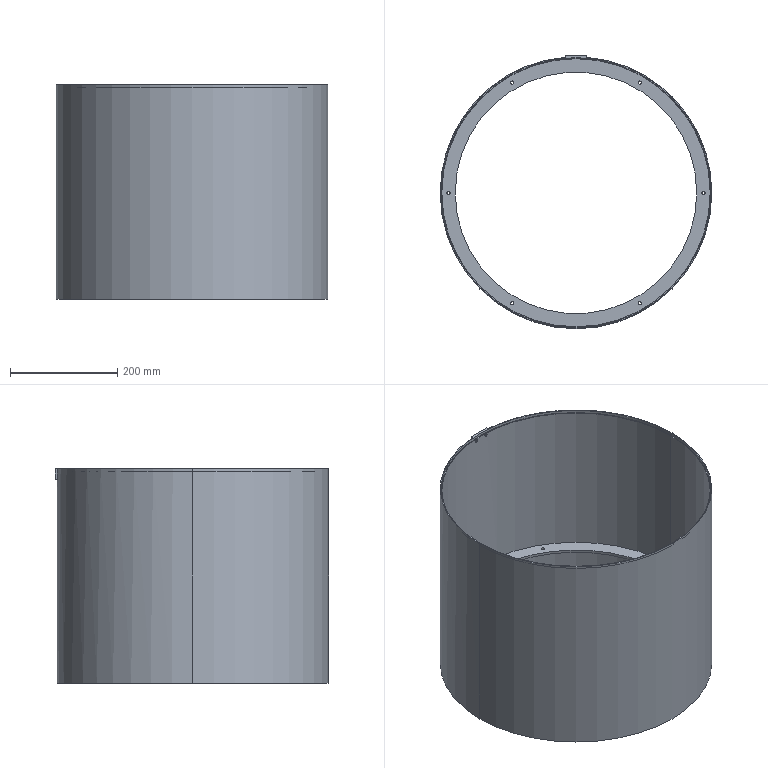Part | SolidWorks | features ICE 6, CirPattern 1, Extrusion 1 | 1 solid | 35 faces | box 506 x 509 x 400 mm | volume 2072487 mm3 | cylinder 26 | plane 9 | commonest cylinder face diameters 6 x12 5.21 x4 500 x4 450 x2 503 x2 506 x2
STEP:
#1=CARTESIAN_POINT('',(-251.5,0.,395.));
#2=VERTEX_POINT('',#1);
#3=CARTESIAN_POINT('',(251.5,0.,395.));
#4=VERTEX_POINT('',#3);
#5=CARTESIAN_POINT('',(0.,0.,395.));
#6=DIRECTION('',(0.,0.,1.));
#7=DIRECTION('',(1.,0.,0.));
#8=AXIS2_PLACEMENT_3D('',#5,#6,#7);
#9=CIRCLE('',#8,251.5);
#10=EDGE_CURVE('',#2,#4,#9,.T.);
#11=ORIENTED_EDGE('',*,*,#10,.F.);
#12=CARTESIAN_POINT('',(-251.5,0.,400.));
#13=VERTEX_POINT('',#12);
#14=CARTESIAN_POINT('',(-251.5,0.,395.));
#15=DIRECTION('',(0.,0.,1.));
#16=VECTOR('',#15,1000.);
#17=LINE('',#14,#16);
#18=EDGE_CURVE('',#2,#13,#17,.T.);
#19=ORIENTED_EDGE('',*,*,#18,.T.);
#20=CARTESIAN_POINT('',(251.5,0.,400.));
#21=VERTEX_POINT('',#20);
#22=CARTESIAN_POINT('',(0.,0.,400.));
#23=DIRECTION('',(0.,0.,1.));
#24=DIRECTION('',(1.,0.,0.));
#25=AXIS2_PLACEMENT_3D('',#22,#23,#24);
#26=CIRCLE('',#25,251.5);
#27=EDGE_CURVE('',#13,#21,#26,.T.);
#28=ORIENTED_EDGE('',*,*,#27,.T.);
#29=CARTESIAN_POINT('',(251.5,0.,395.));
#30=DIRECTION('',(0.,0.,1.));
#31=VECTOR('',#30,1000.);
#32=LINE('',#29,#31);
#33=EDGE_CURVE('',#4,#21,#32,.T.);
#34=ORIENTED_EDGE('',*,*,#33,.F.);
#35=EDGE_LOOP('',(#11,#19,#28,#34));
#36=FACE_OUTER_BOUND('',#35,.T.);
#37=CARTESIAN_POINT('',(0.,0.,395.));
#38=DIRECTION('',(0.,0.,1.));
#39=DIRECTION('',(1.,0.,0.));
#40=AXIS2_PLACEMENT_3D('',#37,#38,#39);
#41=CYLINDRICAL_SURFACE('',#40,251.5);
#42=ADVANCED_FACE('',(#36),#41,.F.);
#43=CARTESIAN_POINT('',(12.5,249.687,387.395));
#44=VERTEX_POINT('',#43);
#45=CARTESIAN_POINT('',(12.5,249.687,392.605));
#46=VERTEX_POINT('',#45);
#47=CARTESIAN_POINT('',(12.5,249.687,387.395));
#48=CARTESIAN_POINT('',(12.33,249.696,387.395));
#49=CARTESIAN_POINT('',(12.161,249.704,387.412));
#50=CARTESIAN_POINT('',(11.826,249.72,387.478));
#51=CARTESIAN_POINT('',(11.661,249.728,387.528));
#52=CARTESIAN_POINT('',(11.191,249.75,387.722));
#53=CARTESIAN_POINT('',(10.9,249.762,387.916));
#54=CARTESIAN_POINT('',(10.54,249.778,388.276));
#55=CARTESIAN_POINT('',(10.43,249.782,388.41));
#56=CARTESIAN_POINT('',(10.24,249.79,388.693));
#57=CARTESIAN_POINT('',(10.16,249.793,388.843));
#58=CARTESIAN_POINT('',(10.029,249.799,389.158));
#59=CARTESIAN_POINT('',(9.979,249.801,389.324));
#60=CARTESIAN_POINT('',(9.912,249.803,389.657));
#61=CARTESIAN_POINT('',(9.895,249.804,389.826));
#62=CARTESIAN_POINT('',(9.895,249.804,390.17));
#63=CARTESIAN_POINT('',(9.912,249.803,390.34));
#64=CARTESIAN_POINT('',(9.978,249.801,390.673));
#65=CARTESIAN_POINT('',(10.028,249.799,390.838));
#66=CARTESIAN_POINT('',(10.158,249.794,391.154));
#67=CARTESIAN_POINT('',(10.238,249.79,391.304));
#68=CARTESIAN_POINT('',(10.427,249.782,391.587));
#69=CARTESIAN_POINT('',(10.537,249.778,391.721));
#70=CARTESIAN_POINT('',(10.777,249.768,391.961));
#71=CARTESIAN_POINT('',(10.908,249.762,392.069));
#72=CARTESIAN_POINT('',(11.193,249.749,392.26));
#73=CARTESIAN_POINT('',(11.345,249.743,392.341));
#74=CARTESIAN_POINT('',(11.814,249.721,392.536));
#75=CARTESIAN_POINT('',(12.156,249.705,392.605));
#76=CARTESIAN_POINT('',(12.5,249.687,392.605));
#77=B_SPLINE_CURVE_WITH_KNOTS('',3,(#47,#48,#49,#50,#51,#52,#53,#54,#55,#56,#57,#58,#59,#60,#61,#62,#63,#64,#65,#66,#67,#68,#69,#70,#71,#72,#73,#74,#75,#76),.UNSPECIFIED.,.F.,.F.,(4,2,2,2,2,2,2,2,2,2,2,2,2,2,4),(0.00815,0.008659,0.009168,0.01019,0.0107,0.01121,0.01171,0.01222,0.01273,0.01324,0.01375,0.01426,0.01477,0.01528,0.0163),.UNSPECIFIED.);
#78=EDGE_CURVE('',#44,#46,#77,.T.);
#79=ORIENTED_EDGE('',*,*,#78,.F.);
#80=CARTESIAN_POINT('',(12.5,256.,387.395));
#81=VERTEX_POINT('',#80);
#82=CARTESIAN_POINT('',(12.5,-253.001,387.395));
#83=DIRECTION('',(0.,1.,0.));
#84=VECTOR('',#83,1000.);
#85=LINE('',#82,#84);
#86=EDGE_CURVE('',#44,#81,#85,.T.);
#87=ORIENTED_EDGE('',*,*,#86,.T.);
#88=CARTESIAN_POINT('',(12.5,256.,392.605));
#89=VERTEX_POINT('',#88);
#90=CARTESIAN_POINT('',(12.5,256.,390.));
#91=DIRECTION('',(0.,1.,0.));
#92=DIRECTION('',(0.,0.,-1.));
#93=AXIS2_PLACEMENT_3D('',#90,#91,#92);
#94=CIRCLE('',#93,2.605);
#95=EDGE_CURVE('',#81,#89,#94,.T.);
#96=ORIENTED_EDGE('',*,*,#95,.T.);
#97=CARTESIAN_POINT('',(12.5,-253.001,392.605));
#98=DIRECTION('',(0.,1.,0.));
#99=VECTOR('',#98,1000.);
#100=LINE('',#97,#99);
#101=EDGE_CURVE('',#46,#89,#100,.T.);
#102=ORIENTED_EDGE('',*,*,#101,.F.);
#103=EDGE_LOOP('',(#79,#87,#96,#102));
#104=FACE_OUTER_BOUND('',#103,.T.);
#105=CARTESIAN_POINT('',(12.5,-253.001,390.));
#106=DIRECTION('',(0.,1.,0.));
#107=DIRECTION('',(0.,0.,1.));
#108=AXIS2_PLACEMENT_3D('',#105,#106,#107);
#109=CYLINDRICAL_SURFACE('',#108,2.605);
#110=ADVANCED_FACE('',(#104),#109,.F.);
#111=CARTESIAN_POINT('',(-12.5,249.687,387.395));
#112=VERTEX_POINT('',#111);
#113=CARTESIAN_POINT('',(-12.5,249.687,392.605));
#114=VERTEX_POINT('',#113);
#115=CARTESIAN_POINT('',(-12.5,249.687,387.395));
#116=CARTESIAN_POINT('',(-12.67,249.679,387.395));
#117=CARTESIAN_POINT('',(-12.839,249.67,387.412));
#118=CARTESIAN_POINT('',(-13.174,249.653,387.478));
#119=CARTESIAN_POINT('',(-13.339,249.644,387.528));
#120=CARTESIAN_POINT('',(-13.809,249.619,387.722));
#121=CARTESIAN_POINT('',(-14.1,249.602,387.916));
#122=CARTESIAN_POINT('',(-14.46,249.581,388.276));
#123=CARTESIAN_POINT('',(-14.57,249.575,388.41));
#124=CARTESIAN_POINT('',(-14.76,249.564,388.693));
#125=CARTESIAN_POINT('',(-14.84,249.559,388.843));
#126=CARTESIAN_POINT('',(-14.971,249.551,389.158));
#127=CARTESIAN_POINT('',(-15.021,249.548,389.323));
#128=CARTESIAN_POINT('',(-15.088,249.544,389.657));
#129=CARTESIAN_POINT('',(-15.105,249.543,389.826));
#130=CARTESIAN_POINT('',(-15.105,249.543,390.17));
#131=CARTESIAN_POINT('',(-15.088,249.544,390.34));
#132=CARTESIAN_POINT('',(-15.022,249.548,390.673));
#133=CARTESIAN_POINT('',(-14.972,249.551,390.838));
#134=CARTESIAN_POINT('',(-14.842,249.559,391.154));
#135=CARTESIAN_POINT('',(-14.762,249.564,391.304));
#136=CARTESIAN_POINT('',(-14.573,249.575,391.587));
#137=CARTESIAN_POINT('',(-14.463,249.581,391.721));
#138=CARTESIAN_POINT('',(-14.222,249.595,391.962));
#139=CARTESIAN_POINT('',(-14.091,249.603,392.069));
#140=CARTESIAN_POINT('',(-13.807,249.618,392.26));
#141=CARTESIAN_POINT('',(-13.655,249.627,392.341));
#142=CARTESIAN_POINT('',(-13.186,249.652,392.536));
#143=CARTESIAN_POINT('',(-12.844,249.67,392.605));
#144=CARTESIAN_POINT('',(-12.5,249.687,392.605));
#145=B_SPLINE_CURVE_WITH_KNOTS('',3,(#115,#116,#117,#118,#119,#120,#121,#122,#123,#124,#125,#126,#127,#128,#129,#130,#131,#132,#133,#134,#135,#136,#137,#138,#139,#140,#141,#142,#143,#144),.UNSPECIFIED.,.F.,.F.,(4,2,2,2,2,2,2,2,2,2,2,2,2,2,4),(0.008148,0.008658,0.009167,0.01019,0.01069,0.0112,0.01171,0.01222,0.01273,0.01324,0.01375,0.01426,0.01477,0.01528,0.0163),.UNSPECIFIED.);
#146=EDGE_CURVE('',#112,#114,#145,.T.);
#147=ORIENTED_EDGE('',*,*,#146,.F.);
#148=CARTESIAN_POINT('',(-12.5,256.,387.395));
#149=VERTEX_POINT('',#148);
#150=CARTESIAN_POINT('',(-12.5,-253.001,387.395));
#151=DIRECTION('',(0.,1.,0.));
#152=VECTOR('',#151,1000.);
#153=LINE('',#150,#152);
#154=EDGE_CURVE('',#112,#149,#153,.T.);
#155=ORIENTED_EDGE('',*,*,#154,.T.);
#156=CARTESIAN_POINT('',(-12.5,256.,392.605));
#157=VERTEX_POINT('',#156);
#158=CARTESIAN_POINT('',(-12.5,256.,390.));
#159=DIRECTION('',(0.,1.,0.));
#160=DIRECTION('',(0.,0.,1.));
#161=AXIS2_PLACEMENT_3D('',#158,#159,#160);
#162=CIRCLE('',#161,2.605);
#163=EDGE_CURVE('',#149,#157,#162,.T.);
#164=ORIENTED_EDGE('',*,*,#163,.T.);
#165=CARTESIAN_POINT('',(-12.5,-253.001,392.605));
#166=DIRECTION('',(0.,1.,0.));
#167=VECTOR('',#166,1000.);
#168=LINE('',#165,#167);
#169=EDGE_CURVE('',#114,#157,#168,.T.);
#170=ORIENTED_EDGE('',*,*,#169,.F.);
#171=EDGE_LOOP('',(#147,#155,#164,#170));
#172=FACE_OUTER_BOUND('',#171,.T.);
#173=CARTESIAN_POINT('',(-12.5,-253.001,390.));
#174=DIRECTION('',(0.,1.,0.));
#175=DIRECTION('',(0.,0.,1.));
#176=AXIS2_PLACEMENT_3D('',#173,#174,#175);
#177=CYLINDRICAL_SURFACE('',#176,2.605);
#178=ADVANCED_FACE('',(#172),#177,.F.);
#179=CARTESIAN_POINT('',(121.75,205.681,100.));
#180=VERTEX_POINT('',#179);
#181=CARTESIAN_POINT('',(115.75,205.681,100.));
#182=VERTEX_POINT('',#181);
#183=CARTESIAN_POINT('',(118.75,205.681,100.));
#184=DIRECTION('',(0.,0.,-1.));
#185=DIRECTION('',(-1.,0.,0.));
#186=AXIS2_PLACEMENT_3D('',#183,#184,#185);
#187=CIRCLE('',#186,3.);
#188=EDGE_CURVE('',#180,#182,#187,.T.);
#189=ORIENTED_EDGE('',*,*,#188,.F.);
#190=CARTESIAN_POINT('',(121.75,205.681,95.));
#191=VERTEX_POINT('',#190);
#192=CARTESIAN_POINT('',(121.75,205.681,115.));
#193=DIRECTION('',(0.,0.,-1.));
#194=VECTOR('',#193,1000.);
#195=LINE('',#192,#194);
#196=EDGE_CURVE('',#180,#191,#195,.T.);
#197=ORIENTED_EDGE('',*,*,#196,.T.);
#198=CARTESIAN_POINT('',(115.75,205.681,95.));
#199=VERTEX_POINT('',#198);
#200=CARTESIAN_POINT('',(118.75,205.681,95.));
#201=DIRECTION('',(0.,0.,-1.));
#202=DIRECTION('',(0.5,0.866,0.));
#203=AXIS2_PLACEMENT_3D('',#200,#201,#202);
#204=CIRCLE('',#203,3.);
#205=EDGE_CURVE('',#191,#199,#204,.T.);
#206=ORIENTED_EDGE('',*,*,#205,.T.);
#207=CARTESIAN_POINT('',(115.75,205.681,115.));
#208=DIRECTION('',(0.,0.,-1.));
#209=VECTOR('',#208,1000.);
#210=LINE('',#207,#209);
#211=EDGE_CURVE('',#182,#199,#210,.T.);
#212=ORIENTED_EDGE('',*,*,#211,.F.);
#213=EDGE_LOOP('',(#189,#197,#206,#212));
#214=FACE_OUTER_BOUND('',#213,.T.);
#215=CARTESIAN_POINT('',(118.75,205.681,115.));
#216=DIRECTION('',(0.,0.,-1.));
#217=DIRECTION('',(-1.,0.,0.));
#218=AXIS2_PLACEMENT_3D('',#215,#216,#217);
#219=CYLINDRICAL_SURFACE('',#218,3.);
#220=ADVANCED_FACE('',(#214),#219,.F.);
#221=CARTESIAN_POINT('',(240.5,0.,100.));
#222=VERTEX_POINT('',#221);
#223=CARTESIAN_POINT('',(234.5,0.,100.));
#224=VERTEX_POINT('',#223);
#225=CARTESIAN_POINT('',(237.5,0.,100.));
#226=DIRECTION('',(0.,0.,-1.));
#227=DIRECTION('',(-1.,0.,0.));
#228=AXIS2_PLACEMENT_3D('',#225,#226,#227);
#229=CIRCLE('',#228,3.);
#230=EDGE_CURVE('',#222,#224,#229,.T.);
#231=ORIENTED_EDGE('',*,*,#230,.F.);
#232=CARTESIAN_POINT('',(240.5,0.,95.));
#233=VERTEX_POINT('',#232);
#234=CARTESIAN_POINT('',(240.5,0.,115.));
#235=DIRECTION('',(0.,0.,-1.));
#236=VECTOR('',#235,1000.);
#237=LINE('',#234,#236);
#238=EDGE_CURVE('',#222,#233,#237,.T.);
#239=ORIENTED_EDGE('',*,*,#238,.T.);
#240=CARTESIAN_POINT('',(234.5,0.,95.));
#241=VERTEX_POINT('',#240);
#242=CARTESIAN_POINT('',(237.5,0.,95.));
#243=DIRECTION('',(0.,0.,-1.));
#244=DIRECTION('',(1.,0.,0.));
#245=AXIS2_PLACEMENT_3D('',#242,#243,#244);
#246=CIRCLE('',#245,3.);
#247=EDGE_CURVE('',#233,#241,#246,.T.);
#248=ORIENTED_EDGE('',*,*,#247,.T.);
#249=CARTESIAN_POINT('',(234.5,0.,115.));
#250=DIRECTION('',(0.,0.,-1.));
#251=VECTOR('',#250,1000.);
#252=LINE('',#249,#251);
#253=EDGE_CURVE('',#224,#241,#252,.T.);
#254=ORIENTED_EDGE('',*,*,#253,.F.);
#255=EDGE_LOOP('',(#231,#239,#248,#254));
#256=FACE_OUTER_BOUND('',#255,.T.);
#257=CARTESIAN_POINT('',(237.5,0.,115.));
#258=DIRECTION('',(0.,0.,-1.));
#259=DIRECTION('',(-1.,0.,0.));
#260=AXIS2_PLACEMENT_3D('',#257,#258,#259);
#261=CYLINDRICAL_SURFACE('',#260,3.);
#262=ADVANCED_FACE('',(#256),#261,.F.);
#263=CARTESIAN_POINT('',(121.75,-205.681,100.));
#264=VERTEX_POINT('',#263);
#265=CARTESIAN_POINT('',(115.75,-205.681,100.));
#266=VERTEX_POINT('',#265);
#267=CARTESIAN_POINT('',(118.75,-205.681,100.));
#268=DIRECTION('',(0.,0.,-1.));
#269=DIRECTION('',(-1.,0.,0.));
#270=AXIS2_PLACEMENT_3D('',#267,#268,#269);
#271=CIRCLE('',#270,3.);
#272=EDGE_CURVE('',#264,#266,#271,.T.);
#273=ORIENTED_EDGE('',*,*,#272,.F.);
#274=CARTESIAN_POINT('',(121.75,-205.681,95.));
#275=VERTEX_POINT('',#274);
#276=CARTESIAN_POINT('',(121.75,-205.681,115.));
#277=DIRECTION('',(0.,0.,-1.));
#278=VECTOR('',#277,1000.);
#279=LINE('',#276,#278);
#280=EDGE_CURVE('',#264,#275,#279,.T.);
#281=ORIENTED_EDGE('',*,*,#280,.T.);
#282=CARTESIAN_POINT('',(115.75,-205.681,95.));
#283=VERTEX_POINT('',#282);
#284=CARTESIAN_POINT('',(118.75,-205.681,95.));
#285=DIRECTION('',(0.,0.,-1.));
#286=DIRECTION('',(0.5,-0.866,0.));
#287=AXIS2_PLACEMENT_3D('',#284,#285,#286);
#288=CIRCLE('',#287,3.);
#289=EDGE_CURVE('',#275,#283,#288,.T.);
#290=ORIENTED_EDGE('',*,*,#289,.T.);
#291=CARTESIAN_POINT('',(115.75,-205.681,115.));
#292=DIRECTION('',(0.,0.,-1.));
#293=VECTOR('',#292,1000.);
#294=LINE('',#291,#293);
#295=EDGE_CURVE('',#266,#283,#294,.T.);
#296=ORIENTED_EDGE('',*,*,#295,.F.);
#297=EDGE_LOOP('',(#273,#281,#290,#296));
#298=FACE_OUTER_BOUND('',#297,.T.);
#299=CARTESIAN_POINT('',(118.75,-205.681,115.));
#300=DIRECTION('',(0.,0.,-1.));
#301=DIRECTION('',(-1.,0.,0.));
#302=AXIS2_PLACEMENT_3D('',#299,#300,#301);
#303=CYLINDRICAL_SURFACE('',#302,3.);
#304=ADVANCED_FACE('',(#298),#303,.F.);
#305=CARTESIAN_POINT('',(-115.75,-205.681,100.));
#306=VERTEX_POINT('',#305);
#307=CARTESIAN_POINT('',(-121.75,-205.681,100.));
#308=VERTEX_POINT('',#307);
#309=CARTESIAN_POINT('',(-118.75,-205.681,100.));
#310=DIRECTION('',(0.,0.,-1.));
#311=DIRECTION('',(-1.,0.,0.));
#312=AXIS2_PLACEMENT_3D('',#309,#310,#311);
#313=CIRCLE('',#312,3.);
#314=EDGE_CURVE('',#306,#308,#313,.T.);
#315=ORIENTED_EDGE('',*,*,#314,.F.);
#316=CARTESIAN_POINT('',(-115.75,-205.681,95.));
#317=VERTEX_POINT('',#316);
#318=CARTESIAN_POINT('',(-115.75,-205.681,115.));
#319=DIRECTION('',(0.,0.,-1.));
#320=VECTOR('',#319,1000.);
#321=LINE('',#318,#320);
#322=EDGE_CURVE('',#306,#317,#321,.T.);
#323=ORIENTED_EDGE('',*,*,#322,.T.);
#324=CARTESIAN_POINT('',(-121.75,-205.681,95.));
#325=VERTEX_POINT('',#324);
#326=CARTESIAN_POINT('',(-118.75,-205.681,95.));
#327=DIRECTION('',(0.,0.,-1.));
#328=DIRECTION('',(-0.5,-0.866,0.));
#329=AXIS2_PLACEMENT_3D('',#326,#327,#328);
#330=CIRCLE('',#329,3.);
#331=EDGE_CURVE('',#317,#325,#330,.T.);
#332=ORIENTED_EDGE('',*,*,#331,.T.);
#333=CARTESIAN_POINT('',(-121.75,-205.681,115.));
#334=DIRECTION('',(0.,0.,-1.));
#335=VECTOR('',#334,1000.);
#336=LINE('',#333,#335);
#337=EDGE_CURVE('',#308,#325,#336,.T.);
#338=ORIENTED_EDGE('',*,*,#337,.F.);
#339=EDGE_LOOP('',(#315,#323,#332,#338));
#340=FACE_OUTER_BOUND('',#339,.T.);
#341=CARTESIAN_POINT('',(-118.75,-205.681,115.));
#342=DIRECTION('',(0.,0.,-1.));
#343=DIRECTION('',(-1.,0.,0.));
#344=AXIS2_PLACEMENT_3D('',#341,#342,#343);
#345=CYLINDRICAL_SURFACE('',#344,3.);
#346=ADVANCED_FACE('',(#340),#345,.F.);
#347=CARTESIAN_POINT('',(-115.75,205.681,100.));
#348=VERTEX_POINT('',#347);
#349=CARTESIAN_POINT('',(-121.75,205.681,100.));
#350=VERTEX_POINT('',#349);
#351=CARTESIAN_POINT('',(-118.75,205.681,100.));
#352=DIRECTION('',(0.,0.,-1.));
#353=DIRECTION('',(-1.,0.,0.));
#354=AXIS2_PLACEMENT_3D('',#351,#352,#353);
#355=CIRCLE('',#354,3.);
#356=EDGE_CURVE('',#348,#350,#355,.T.);
#357=ORIENTED_EDGE('',*,*,#356,.F.);
#358=CARTESIAN_POINT('',(-115.75,205.681,95.));
#359=VERTEX_POINT('',#358);
#360=CARTESIAN_POINT('',(-115.75,205.681,115.));
#361=DIRECTION('',(0.,0.,-1.));
#362=VECTOR('',#361,1000.);
#363=LINE('',#360,#362);
#364=EDGE_CURVE('',#348,#359,#363,.T.);
#365=ORIENTED_EDGE('',*,*,#364,.T.);
#366=CARTESIAN_POINT('',(-121.75,205.681,95.));
#367=VERTEX_POINT('',#366);
#368=CARTESIAN_POINT('',(-118.75,205.681,95.));
#369=DIRECTION('',(0.,0.,-1.));
#370=DIRECTION('',(-0.5,0.866,0.));
#371=AXIS2_PLACEMENT_3D('',#368,#369,#370);
#372=CIRCLE('',#371,3.);
#373=EDGE_CURVE('',#359,#367,#372,.T.);
#374=ORIENTED_EDGE('',*,*,#373,.T.);
#375=CARTESIAN_POINT('',(-121.75,205.681,115.));
#376=DIRECTION('',(0.,0.,-1.));
#377=VECTOR('',#376,1000.);
#378=LINE('',#375,#377);
#379=EDGE_CURVE('',#350,#367,#378,.T.);
#380=ORIENTED_EDGE('',*,*,#379,.F.);
#381=EDGE_LOOP('',(#357,#365,#374,#380));
#382=FACE_OUTER_BOUND('',#381,.T.);
#383=CARTESIAN_POINT('',(-118.75,205.681,115.));
#384=DIRECTION('',(0.,0.,-1.));
#385=DIRECTION('',(-1.,0.,0.));
#386=AXIS2_PLACEMENT_3D('',#383,#384,#385);
#387=CYLINDRICAL_SURFACE('',#386,3.);
#388=ADVANCED_FACE('',(#382),#387,.F.);
#389=CARTESIAN_POINT('',(-234.5,0.,100.));
#390=VERTEX_POINT('',#389);
#391=CARTESIAN_POINT('',(-240.5,0.,100.));
#392=VERTEX_POINT('',#391);
#393=CARTESIAN_POINT('',(-237.5,0.,100.));
#394=DIRECTION('',(0.,0.,-1.));
#395=DIRECTION('',(-1.,0.,0.));
#396=AXIS2_PLACEMENT_3D('',#393,#394,#395);
#397=CIRCLE('',#396,3.);
#398=EDGE_CURVE('',#390,#392,#397,.T.);
#399=ORIENTED_EDGE('',*,*,#398,.F.);
#400=CARTESIAN_POINT('',(-234.5,0.,95.));
#401=VERTEX_POINT('',#400);
#402=CARTESIAN_POINT('',(-234.5,0.,115.));
#403=DIRECTION('',(0.,0.,-1.));
#404=VECTOR('',#403,1000.);
#405=LINE('',#402,#404);
#406=EDGE_CURVE('',#390,#401,#405,.T.);
#407=ORIENTED_EDGE('',*,*,#406,.T.);
#408=CARTESIAN_POINT('',(-240.5,0.,95.));
#409=VERTEX_POINT('',#408);
#410=CARTESIAN_POINT('',(-237.5,0.,95.));
#411=DIRECTION('',(0.,0.,-1.));
#412=DIRECTION('',(-1.,0.,0.));
#413=AXIS2_PLACEMENT_3D('',#410,#411,#412);
#414=CIRCLE('',#413,3.);
#415=EDGE_CURVE('',#401,#409,#414,.T.);
#416=ORIENTED_EDGE('',*,*,#415,.T.);
#417=CARTESIAN_POINT('',(-240.5,0.,115.));
#418=DIRECTION('',(0.,0.,-1.));
#419=VECTOR('',#418,1000.);
#420=LINE('',#417,#419);
#421=EDGE_CURVE('',#392,#409,#420,.T.);
#422=ORIENTED_EDGE('',*,*,#421,.F.);
#423=EDGE_LOOP('',(#399,#407,#416,#422));
#424=FACE_OUTER_BOUND('',#423,.T.);
#425=CARTESIAN_POINT('',(-237.5,0.,115.));
#426=DIRECTION('',(0.,0.,-1.));
#427=DIRECTION('',(-1.,0.,0.));
#428=AXIS2_PLACEMENT_3D('',#425,#426,#427);
#429=CYLINDRICAL_SURFACE('',#428,3.);
#430=ADVANCED_FACE('',(#424),#429,.F.);
#431=CARTESIAN_POINT('',(225.,0.,95.));
#432=VERTEX_POINT('',#431);
#433=CARTESIAN_POINT('',(-225.,0.,95.));
#434=VERTEX_POINT('',#433);
#435=CARTESIAN_POINT('',(0.,0.,95.));
#436=DIRECTION('',(0.,0.,-1.));
#437=DIRECTION('',(-1.,0.,0.));
#438=AXIS2_PLACEMENT_3D('',#435,#436,#437);
#439=CIRCLE('',#438,225.);
#440=EDGE_CURVE('',#432,#434,#439,.T.);
#441=ORIENTED_EDGE('',*,*,#440,.T.);
#442=CARTESIAN_POINT('',(-225.,0.,100.));
#443=VERTEX_POINT('',#442);
#444=CARTESIAN_POINT('',(-225.,0.,95.));
#445=DIRECTION('',(0.,0.,1.));
#446=VECTOR('',#445,1000.);
#447=LINE('',#444,#446);
#448=EDGE_CURVE('',#434,#443,#447,.T.);
#449=ORIENTED_EDGE('',*,*,#448,.T.);
#450=CARTESIAN_POINT('',(225.,0.,100.));
#451=VERTEX_POINT('',#450);
#452=CARTESIAN_POINT('',(0.,0.,100.));
#453=DIRECTION('',(0.,0.,-1.));
#454=DIRECTION('',(-1.,0.,0.));
#455=AXIS2_PLACEMENT_3D('',#452,#453,#454);
#456=CIRCLE('',#455,225.);
#457=EDGE_CURVE('',#451,#443,#456,.T.);
#458=ORIENTED_EDGE('',*,*,#457,.F.);
#459=CARTESIAN_POINT('',(225.,0.,95.));
#460=DIRECTION('',(0.,0.,1.));
#461=VECTOR('',#460,1000.);
#462=LINE('',#459,#461);
#463=EDGE_CURVE('',#432,#451,#462,.T.);
#464=ORIENTED_EDGE('',*,*,#463,.F.);
#465=EDGE_LOOP('',(#441,#449,#458,#464));
#466=FACE_OUTER_BOUND('',#465,.T.);
#467=CARTESIAN_POINT('',(0.,0.,95.));
#468=DIRECTION('',(0.,0.,1.));
#469=DIRECTION('',(1.,0.,0.));
#470=AXIS2_PLACEMENT_3D('',#467,#468,#469);
#471=CYLINDRICAL_SURFACE('',#470,225.);
#472=ADVANCED_FACE('',(#466),#471,.F.);
#473=CARTESIAN_POINT('',(250.,0.,95.));
#474=VERTEX_POINT('',#473);
#475=CARTESIAN_POINT('',(-250.,0.,95.));
#476=VERTEX_POINT('',#475);
#477=CARTESIAN_POINT('',(0.,0.,95.));
#478=DIRECTION('',(0.,0.,-1.));
#479=DIRECTION('',(-1.,0.,0.));
#480=AXIS2_PLACEMENT_3D('',#477,#478,#479);
#481=CIRCLE('',#480,250.);
#482=EDGE_CURVE('',#474,#476,#481,.T.);
#483=ORIENTED_EDGE('',*,*,#482,.F.);
#484=CARTESIAN_POINT('',(250.,0.,0.));
#485=VERTEX_POINT('',#484);
#486=CARTESIAN_POINT('',(250.,0.,400.));
#487=DIRECTION('',(0.,0.,-1.));
#488=VECTOR('',#487,1000.);
#489=LINE('',#486,#488);
#490=EDGE_CURVE('',#474,#485,#489,.T.);
#491=ORIENTED_EDGE('',*,*,#490,.T.);
#492=CARTESIAN_POINT('',(-250.,0.,0.));
#493=VERTEX_POINT('',#492);
#494=CARTESIAN_POINT('',(0.,0.,0.));
#495=DIRECTION('',(0.,0.,1.));
#496=DIRECTION('',(1.,0.,0.));
#497=AXIS2_PLACEMENT_3D('',#494,#495,#496);
#498=CIRCLE('',#497,250.);
#499=EDGE_CURVE('',#493,#485,#498,.T.);
#500=ORIENTED_EDGE('',*,*,#499,.F.);
#501=CARTESIAN_POINT('',(-250.,0.,400.));
#502=DIRECTION('',(0.,0.,-1.));
#503=VECTOR('',#502,1000.);
#504=LINE('',#501,#503);
#505=EDGE_CURVE('',#476,#493,#504,.T.);
#506=ORIENTED_EDGE('',*,*,#505,.F.);
#507=EDGE_LOOP('',(#483,#491,#500,#506));
#508=FACE_OUTER_BOUND('',#507,.T.);
#509=CARTESIAN_POINT('',(0.,0.,400.));
#510=DIRECTION('',(0.,0.,-1.));
#511=DIRECTION('',(-1.,0.,0.));
#512=AXIS2_PLACEMENT_3D('',#509,#510,#511);
#513=CYLINDRICAL_SURFACE('',#512,250.);
#514=ADVANCED_FACE('',(#508),#513,.F.);
#515=CARTESIAN_POINT('',(253.,0.,400.));
#516=VERTEX_POINT('',#515);
#517=CARTESIAN_POINT('',(20.,252.208,400.));
#518=VERTEX_POINT('',#517);
#519=CARTESIAN_POINT('',(0.,0.,400.));
#520=DIRECTION('',(0.,0.,1.));
#521=DIRECTION('',(1.,0.,0.));
#522=AXIS2_PLACEMENT_3D('',#519,#520,#521);
#523=CIRCLE('',#522,253.);
#524=EDGE_CURVE('',#516,#518,#523,.T.);
#525=ORIENTED_EDGE('',*,*,#524,.F.);
#526=CARTESIAN_POINT('',(253.,0.,0.));
#527=VERTEX_POINT('',#526);
#528=CARTESIAN_POINT('',(253.,0.,400.));
#529=DIRECTION('',(0.,0.,-1.));
#530=VECTOR('',#529,1000.);
#531=LINE('',#528,#530);
#532=EDGE_CURVE('',#516,#527,#531,.T.);
#533=ORIENTED_EDGE('',*,*,#532,.T.);
#534=CARTESIAN_POINT('',(-253.,0.,0.));
#535=VERTEX_POINT('',#534);
#536=CARTESIAN_POINT('',(0.,0.,0.));
#537=DIRECTION('',(0.,0.,1.));
#538=DIRECTION('',(1.,0.,0.));
#539=AXIS2_PLACEMENT_3D('',#536,#537,#538);
#540=CIRCLE('',#539,253.);
#541=EDGE_CURVE('',#527,#535,#540,.T.);
#542=ORIENTED_EDGE('',*,*,#541,.T.);
#543=CARTESIAN_POINT('',(-253.,0.,400.));
#544=VERTEX_POINT('',#543);
#545=CARTESIAN_POINT('',(-253.,0.,400.));
#546=DIRECTION('',(0.,0.,-1.));
#547=VECTOR('',#546,1000.);
#548=LINE('',#545,#547);
#549=EDGE_CURVE('',#544,#535,#548,.T.);
#550=ORIENTED_EDGE('',*,*,#549,.F.);
#551=CARTESIAN_POINT('',(-20.,252.208,400.));
#552=VERTEX_POINT('',#551);
#553=CARTESIAN_POINT('',(0.,0.,400.));
#554=DIRECTION('',(0.,0.,1.));
#555=DIRECTION('',(1.,0.,0.));
#556=AXIS2_PLACEMENT_3D('',#553,#554,#555);
#557=CIRCLE('',#556,253.);
#558=EDGE_CURVE('',#552,#544,#557,.T.);
#559=ORIENTED_EDGE('',*,*,#558,.F.);
#560=CARTESIAN_POINT('',(-20.,252.208,380.));
#561=VERTEX_POINT('',#560);
#562=CARTESIAN_POINT('',(-20.,252.208,400.));
#563=DIRECTION('',(0.,0.,1.));
#564=VECTOR('',#563,1000.);
#565=LINE('',#562,#564);
#566=EDGE_CURVE('',#561,#552,#565,.T.);
#567=ORIENTED_EDGE('',*,*,#566,.F.);
#568=CARTESIAN_POINT('',(20.,252.208,380.));
#569=VERTEX_POINT('',#568);
#570=CARTESIAN_POINT('',(0.,0.,380.));
#571=DIRECTION('',(0.,0.,1.));
#572=DIRECTION('',(-1.,0.,0.));
#573=AXIS2_PLACEMENT_3D('',#570,#571,#572);
#574=CIRCLE('',#573,253.);
#575=EDGE_CURVE('',#569,#561,#574,.T.);
#576=ORIENTED_EDGE('',*,*,#575,.F.);
#577=CARTESIAN_POINT('',(20.,252.208,400.));
#578=DIRECTION('',(0.,0.,-1.));
#579=VECTOR('',#578,1000.);
#580=LINE('',#577,#579);
#581=EDGE_CURVE('',#518,#569,#580,.T.);
#582=ORIENTED_EDGE('',*,*,#581,.F.);
#583=EDGE_LOOP('',(#525,#533,#542,#550,#559,#567,#576,#582));
#584=FACE_OUTER_BOUND('',#583,.T.);
#585=CARTESIAN_POINT('',(0.,0.,400.));
#586=DIRECTION('',(0.,0.,-1.));
#587=DIRECTION('',(-1.,0.,0.));
#588=AXIS2_PLACEMENT_3D('',#585,#586,#587);
#589=CYLINDRICAL_SURFACE('',#588,253.);
#590=ADVANCED_FACE('',(#584),#589,.T.);
#591=CARTESIAN_POINT('',(-250.,0.,395.));
#592=VERTEX_POINT('',#591);
#593=CARTESIAN_POINT('',(250.,0.,395.));
#594=VERTEX_POINT('',#593);
#595=CARTESIAN_POINT('',(0.,0.,395.));
#596=DIRECTION('',(0.,0.,1.));
#597=DIRECTION('',(1.,0.,0.));
#598=AXIS2_PLACEMENT_3D('',#595,#596,#597);
#599=CIRCLE('',#598,250.);
#600=EDGE_CURVE('',#592,#594,#599,.T.);
#601=ORIENTED_EDGE('',*,*,#600,.T.);
#602=CARTESIAN_POINT('',(250.,0.,100.));
#603=VERTEX_POINT('',#602);
#604=CARTESIAN_POINT('',(250.,0.,400.));
#605=DIRECTION('',(0.,0.,-1.));
#606=VECTOR('',#605,1000.);
#607=LINE('',#604,#606);
#608=EDGE_CURVE('',#594,#603,#607,.T.);
#609=ORIENTED_EDGE('',*,*,#608,.T.);
#610=CARTESIAN_POINT('',(-250.,0.,100.));
#611=VERTEX_POINT('',#610);
#612=CARTESIAN_POINT('',(0.,0.,100.));
#613=DIRECTION('',(0.,0.,-1.));
#614=DIRECTION('',(-1.,0.,0.));
#615=AXIS2_PLACEMENT_3D('',#612,#613,#614);
#616=CIRCLE('',#615,250.);
#617=EDGE_CURVE('',#603,#611,#616,.T.);
#618=ORIENTED_EDGE('',*,*,#617,.T.);
#619=CARTESIAN_POINT('',(-250.,0.,400.));
#620=DIRECTION('',(0.,0.,-1.));
#621=VECTOR('',#620,1000.);
#622=LINE('',#619,#621);
#623=EDGE_CURVE('',#592,#611,#622,.T.);
#624=ORIENTED_EDGE('',*,*,#623,.F.);
#625=EDGE_LOOP('',(#601,#609,#618,#624));
#626=FACE_OUTER_BOUND('',#625,.T.);
#627=CARTESIAN_POINT('',(0.,0.,400.));
#628=DIRECTION('',(0.,0.,-1.));
#629=DIRECTION('',(-1.,0.,0.));
#630=AXIS2_PLACEMENT_3D('',#627,#628,#629);
#631=CYLINDRICAL_SURFACE('',#630,250.);
#632=ADVANCED_FACE('',(#626),#631,.F.);
#633=ORIENTED_EDGE('',*,*,#608,.F.);
#634=CARTESIAN_POINT('',(0.,0.,395.));
#635=DIRECTION('',(0.,0.,1.));
#636=DIRECTION('',(1.,0.,0.));
#637=AXIS2_PLACEMENT_3D('',#634,#635,#636);
#638=CIRCLE('',#637,250.);
#639=EDGE_CURVE('',#594,#592,#638,.T.);
#640=ORIENTED_EDGE('',*,*,#639,.T.);
#641=ORIENTED_EDGE('',*,*,#623,.T.);
#642=CARTESIAN_POINT('',(0.,0.,100.));
#643=DIRECTION('',(0.,0.,-1.));
#644=DIRECTION('',(-1.,0.,0.));
#645=AXIS2_PLACEMENT_3D('',#642,#643,#644);
#646=CIRCLE('',#645,250.);
#647=EDGE_CURVE('',#611,#603,#646,.T.);
#648=ORIENTED_EDGE('',*,*,#647,.T.);
#649=EDGE_LOOP('',(#633,#640,#641,#648));
#650=FACE_OUTER_BOUND('',#649,.T.);
#651=CARTESIAN_POINT('',(-12.5,249.687,392.605));
#652=CARTESIAN_POINT('',(-12.328,249.696,392.605));
#653=CARTESIAN_POINT('',(-12.159,249.704,392.588));
#654=CARTESIAN_POINT('',(-11.826,249.72,392.522));
#655=CARTESIAN_POINT('',(-11.661,249.728,392.472));
#656=CARTESIAN_POINT('',(-11.345,249.742,392.341));
#657=CARTESIAN_POINT('',(-11.196,249.749,392.261));
#658=CARTESIAN_POINT('',(-10.913,249.762,392.072));
#659=CARTESIAN_POINT('',(-10.778,249.768,391.962));
#660=CARTESIAN_POINT('',(-10.538,249.778,391.722));
#661=CARTESIAN_POINT('',(-10.43,249.782,391.591));
#662=CARTESIAN_POINT('',(-10.24,249.79,391.306));
#663=CARTESIAN_POINT('',(-10.159,249.794,391.154));
#664=CARTESIAN_POINT('',(-10.029,249.799,390.841));
#665=CARTESIAN_POINT('',(-9.979,249.801,390.677));
#666=CARTESIAN_POINT('',(-9.912,249.803,390.34));
#667=CARTESIAN_POINT('',(-9.895,249.804,390.171));
#668=CARTESIAN_POINT('',(-9.895,249.804,389.831));
#669=CARTESIAN_POINT('',(-9.912,249.803,389.658));
#670=CARTESIAN_POINT('',(-9.979,249.801,389.324));
#671=CARTESIAN_POINT('',(-10.028,249.799,389.162));
#672=CARTESIAN_POINT('',(-10.158,249.794,388.846));
#673=CARTESIAN_POINT('',(-10.24,249.79,388.693));
#674=CARTESIAN_POINT('',(-10.429,249.782,388.411));
#675=CARTESIAN_POINT('',(-10.537,249.778,388.28));
#676=CARTESIAN_POINT('',(-10.78,249.768,388.036));
#677=CARTESIAN_POINT('',(-10.912,249.762,387.928));
#678=CARTESIAN_POINT('',(-11.194,249.749,387.74));
#679=CARTESIAN_POINT('',(-11.346,249.742,387.658));
#680=CARTESIAN_POINT('',(-11.662,249.728,387.528));
#681=CARTESIAN_POINT('',(-11.824,249.72,387.479));
#682=CARTESIAN_POINT('',(-12.158,249.704,387.412));
#683=CARTESIAN_POINT('',(-12.33,249.696,387.395));
#684=CARTESIAN_POINT('',(-12.5,249.687,387.395));
#685=B_SPLINE_CURVE_WITH_KNOTS('',3,(#651,#652,#653,#654,#655,#656,#657,#658,#659,#660,#661,#662,#663,#664,#665,#666,#667,#668,#669,#670,#671,#672,#673,#674,#675,#676,#677,#678,#679,#680,#681,#682,#683,#684),.UNSPECIFIED.,.F.,.F.,(4,2,2,2,2,2,2,2,2,2,2,2,2,2,2,2,4),(0.,0.0005093,0.001019,0.001528,0.002037,0.002546,0.003056,0.003565,0.004074,0.004583,0.005093,0.005602,0.006111,0.006621,0.00713,0.007639,0.008148),.UNSPECIFIED.);
#686=EDGE_CURVE('',#114,#112,#685,.T.);
#687=ORIENTED_EDGE('',*,*,#686,.T.);
#688=ORIENTED_EDGE('',*,*,#146,.T.);
#689=EDGE_LOOP('',(#687,#688));
#690=FACE_BOUND('',#689,.T.);
#691=CARTESIAN_POINT('',(12.5,249.687,392.605));
#692=CARTESIAN_POINT('',(12.672,249.679,392.605));
#693=CARTESIAN_POINT('',(12.841,249.67,392.588));
#694=CARTESIAN_POINT('',(13.174,249.653,392.522));
#695=CARTESIAN_POINT('',(13.339,249.644,392.472));
#696=CARTESIAN_POINT('',(13.655,249.627,392.341));
#697=CARTESIAN_POINT('',(13.804,249.619,392.261));
#698=CARTESIAN_POINT('',(14.087,249.603,392.072));
#699=CARTESIAN_POINT('',(14.221,249.595,391.962));
#700=CARTESIAN_POINT('',(14.462,249.581,391.722));
#701=CARTESIAN_POINT('',(14.57,249.575,391.591));
#702=CARTESIAN_POINT('',(14.76,249.564,391.306));
#703=CARTESIAN_POINT('',(14.841,249.559,391.155));
#704=CARTESIAN_POINT('',(14.971,249.551,390.841));
#705=CARTESIAN_POINT('',(15.021,249.548,390.677));
#706=CARTESIAN_POINT('',(15.088,249.544,390.34));
#707=CARTESIAN_POINT('',(15.105,249.543,390.171));
#708=CARTESIAN_POINT('',(15.105,249.543,389.831));
#709=CARTESIAN_POINT('',(15.088,249.544,389.658));
#710=CARTESIAN_POINT('',(15.021,249.548,389.324));
#711=CARTESIAN_POINT('',(14.972,249.551,389.161));
#712=CARTESIAN_POINT('',(14.842,249.559,388.846));
#713=CARTESIAN_POINT('',(14.76,249.564,388.693));
#714=CARTESIAN_POINT('',(14.571,249.575,388.411));
#715=CARTESIAN_POINT('',(14.463,249.581,388.279));
#716=CARTESIAN_POINT('',(14.22,249.595,388.036));
#717=CARTESIAN_POINT('',(14.088,249.603,387.928));
#718=CARTESIAN_POINT('',(13.806,249.619,387.74));
#719=CARTESIAN_POINT('',(13.654,249.627,387.658));
#720=CARTESIAN_POINT('',(13.338,249.644,387.528));
#721=CARTESIAN_POINT('',(13.176,249.653,387.479));
#722=CARTESIAN_POINT('',(12.842,249.67,387.412));
#723=CARTESIAN_POINT('',(12.67,249.679,387.395));
#724=CARTESIAN_POINT('',(12.5,249.687,387.395));
#725=B_SPLINE_CURVE_WITH_KNOTS('',3,(#691,#692,#693,#694,#695,#696,#697,#698,#699,#700,#701,#702,#703,#704,#705,#706,#707,#708,#709,#710,#711,#712,#713,#714,#715,#716,#717,#718,#719,#720,#721,#722,#723,#724),.UNSPECIFIED.,.F.,.F.,(4,2,2,2,2,2,2,2,2,2,2,2,2,2,2,2,4),(0.,0.0005094,0.001019,0.001528,0.002038,0.002547,0.003056,0.003566,0.004075,0.004584,0.005094,0.005603,0.006113,0.006622,0.007131,0.007641,0.00815),.UNSPECIFIED.);
#726=EDGE_CURVE('',#46,#44,#725,.T.);
#727=ORIENTED_EDGE('',*,*,#726,.T.);
#728=ORIENTED_EDGE('',*,*,#78,.T.);
#729=EDGE_LOOP('',(#727,#728));
#730=FACE_BOUND('',#729,.T.);
#731=CARTESIAN_POINT('',(0.,0.,400.));
#732=DIRECTION('',(0.,0.,-1.));
#733=DIRECTION('',(-1.,0.,0.));
#734=AXIS2_PLACEMENT_3D('',#731,#732,#733);
#735=CYLINDRICAL_SURFACE('',#734,250.);
#736=ADVANCED_FACE('',(#650,#690,#730),#735,.F.);
#737=CARTESIAN_POINT('',(0.,0.,400.));
#738=DIRECTION('',(0.,0.,1.));
#739=DIRECTION('',(1.,0.,0.));
#740=AXIS2_PLACEMENT_3D('',#737,#738,#739);
#741=CIRCLE('',#740,251.5);
#742=EDGE_CURVE('',#21,#13,#741,.T.);
#743=ORIENTED_EDGE('',*,*,#742,.F.);
#744=ORIENTED_EDGE('',*,*,#27,.F.);
#745=EDGE_LOOP('',(#743,#744));
#746=FACE_BOUND('',#745,.T.);
#747=ORIENTED_EDGE('',*,*,#558,.T.);
#748=CARTESIAN_POINT('',(0.,0.,400.));
#749=DIRECTION('',(0.,0.,1.));
#750=DIRECTION('',(1.,0.,0.));
#751=AXIS2_PLACEMENT_3D('',#748,#749,#750);
#752=CIRCLE('',#751,253.);
#753=EDGE_CURVE('',#544,#516,#752,.T.);
#754=ORIENTED_EDGE('',*,*,#753,.T.);
#755=ORIENTED_EDGE('',*,*,#524,.T.);
#756=CARTESIAN_POINT('',(20.,256.,400.));
#757=VERTEX_POINT('',#756);
#758=CARTESIAN_POINT('',(20.,-253.001,400.));
#759=DIRECTION('',(0.,1.,0.));
#760=VECTOR('',#759,1000.);
#761=LINE('',#758,#760);
#762=EDGE_CURVE('',#518,#757,#761,.T.);
#763=ORIENTED_EDGE('',*,*,#762,.T.);
#764=CARTESIAN_POINT('',(-20.,256.,400.));
#765=VERTEX_POINT('',#764);
#766=CARTESIAN_POINT('',(-20.,256.,400.));
#767=DIRECTION('',(1.,0.,0.));
#768=VECTOR('',#767,1000.);
#769=LINE('',#766,#768);
#770=EDGE_CURVE('',#765,#757,#769,.T.);
#771=ORIENTED_EDGE('',*,*,#770,.F.);
#772=CARTESIAN_POINT('',(-20.,-253.001,400.));
#773=DIRECTION('',(0.,1.,0.));
#774=VECTOR('',#773,1000.);
#775=LINE('',#772,#774);
#776=EDGE_CURVE('',#552,#765,#775,.T.);
#777=ORIENTED_EDGE('',*,*,#776,.F.);
#778=EDGE_LOOP('',(#747,#754,#755,#763,#771,#777));
#779=FACE_OUTER_BOUND('',#778,.T.);
#780=CARTESIAN_POINT('',(0.,0.,400.));
#781=DIRECTION('',(0.,0.,1.));
#782=DIRECTION('',(1.,0.,0.));
#783=AXIS2_PLACEMENT_3D('',#780,#781,#782);
#784=PLANE('',#783);
#785=ADVANCED_FACE('',(#746,#779),#784,.T.);
#786=CARTESIAN_POINT('',(0.,0.,0.));
#787=DIRECTION('',(0.,0.,1.));
#788=DIRECTION('',(1.,0.,0.));
#789=AXIS2_PLACEMENT_3D('',#786,#787,#788);
#790=CIRCLE('',#789,253.);
#791=EDGE_CURVE('',#535,#527,#790,.T.);
#792=ORIENTED_EDGE('',*,*,#791,.F.);
#793=ORIENTED_EDGE('',*,*,#541,.F.);
#794=EDGE_LOOP('',(#792,#793));
#795=FACE_OUTER_BOUND('',#794,.T.);
#796=ORIENTED_EDGE('',*,*,#499,.T.);
#797=CARTESIAN_POINT('',(0.,0.,0.));
#798=DIRECTION('',(0.,0.,1.));
#799=DIRECTION('',(1.,0.,0.));
#800=AXIS2_PLACEMENT_3D('',#797,#798,#799);
#801=CIRCLE('',#800,250.);
#802=EDGE_CURVE('',#485,#493,#801,.T.);
#803=ORIENTED_EDGE('',*,*,#802,.T.);
#804=EDGE_LOOP('',(#796,#803));
#805=FACE_BOUND('',#804,.T.);
#806=CARTESIAN_POINT('',(0.,0.,0.));
#807=DIRECTION('',(0.,0.,1.));
#808=DIRECTION('',(1.,0.,0.));
#809=AXIS2_PLACEMENT_3D('',#806,#807,#808);
#810=PLANE('',#809);
#811=ADVANCED_FACE('',(#795,#805),#810,.F.);
#812=ORIENTED_EDGE('',*,*,#532,.F.);
#813=ORIENTED_EDGE('',*,*,#753,.F.);
#814=ORIENTED_EDGE('',*,*,#549,.T.);
#815=ORIENTED_EDGE('',*,*,#791,.T.);
#816=EDGE_LOOP('',(#812,#813,#814,#815));
#817=FACE_OUTER_BOUND('',#816,.T.);
#818=CARTESIAN_POINT('',(0.,0.,400.));
#819=DIRECTION('',(0.,0.,-1.));
#820=DIRECTION('',(-1.,0.,0.));
#821=AXIS2_PLACEMENT_3D('',#818,#819,#820);
#822=CYLINDRICAL_SURFACE('',#821,253.);
#823=ADVANCED_FACE('',(#817),#822,.T.);
#824=ORIENTED_EDGE('',*,*,#490,.F.);
#825=CARTESIAN_POINT('',(0.,0.,95.));
#826=DIRECTION('',(0.,0.,-1.));
#827=DIRECTION('',(-1.,0.,0.));
#828=AXIS2_PLACEMENT_3D('',#825,#826,#827);
#829=CIRCLE('',#828,250.);
#830=EDGE_CURVE('',#476,#474,#829,.T.);
#831=ORIENTED_EDGE('',*,*,#830,.F.);
#832=ORIENTED_EDGE('',*,*,#505,.T.);
#833=ORIENTED_EDGE('',*,*,#802,.F.);
#834=EDGE_LOOP('',(#824,#831,#832,#833));
#835=FACE_OUTER_BOUND('',#834,.T.);
#836=CARTESIAN_POINT('',(0.,0.,400.));
#837=DIRECTION('',(0.,0.,-1.));
#838=DIRECTION('',(-1.,0.,0.));
#839=AXIS2_PLACEMENT_3D('',#836,#837,#838);
#840=CYLINDRICAL_SURFACE('',#839,250.);
#841=ADVANCED_FACE('',(#835),#840,.F.);
#842=CARTESIAN_POINT('',(118.75,205.681,95.));
#843=DIRECTION('',(0.,0.,-1.));
#844=DIRECTION('',(0.5,0.866,0.));
#845=AXIS2_PLACEMENT_3D('',#842,#843,#844);
#846=CIRCLE('',#845,3.);
#847=EDGE_CURVE('',#199,#191,#846,.T.);
#848=ORIENTED_EDGE('',*,*,#847,.F.);
#849=ORIENTED_EDGE('',*,*,#205,.F.);
#850=EDGE_LOOP('',(#848,#849));
#851=FACE_BOUND('',#850,.T.);
#852=CARTESIAN_POINT('',(237.5,0.,95.));
#853=DIRECTION('',(0.,0.,-1.));
#854=DIRECTION('',(1.,0.,0.));
#855=AXIS2_PLACEMENT_3D('',#852,#853,#854);
#856=CIRCLE('',#855,3.);
#857=EDGE_CURVE('',#241,#233,#856,.T.);
#858=ORIENTED_EDGE('',*,*,#857,.F.);
#859=ORIENTED_EDGE('',*,*,#247,.F.);
#860=EDGE_LOOP('',(#858,#859));
#861=FACE_BOUND('',#860,.T.);
#862=CARTESIAN_POINT('',(118.75,-205.681,95.));
#863=DIRECTION('',(0.,0.,-1.));
#864=DIRECTION('',(0.5,-0.866,0.));
#865=AXIS2_PLACEMENT_3D('',#862,#863,#864);
#866=CIRCLE('',#865,3.);
#867=EDGE_CURVE('',#283,#275,#866,.T.);
#868=ORIENTED_EDGE('',*,*,#867,.F.);
#869=ORIENTED_EDGE('',*,*,#289,.F.);
#870=EDGE_LOOP('',(#868,#869));
#871=FACE_BOUND('',#870,.T.);
#872=CARTESIAN_POINT('',(-118.75,-205.681,95.));
#873=DIRECTION('',(0.,0.,-1.));
#874=DIRECTION('',(-0.5,-0.866,0.));
#875=AXIS2_PLACEMENT_3D('',#872,#873,#874);
#876=CIRCLE('',#875,3.);
#877=EDGE_CURVE('',#325,#317,#876,.T.);
#878=ORIENTED_EDGE('',*,*,#877,.F.);
#879=ORIENTED_EDGE('',*,*,#331,.F.);
#880=EDGE_LOOP('',(#878,#879));
#881=FACE_BOUND('',#880,.T.);
#882=CARTESIAN_POINT('',(-118.75,205.681,95.));
#883=DIRECTION('',(0.,0.,-1.));
#884=DIRECTION('',(-0.5,0.866,0.));
#885=AXIS2_PLACEMENT_3D('',#882,#883,#884);
#886=CIRCLE('',#885,3.);
#887=EDGE_CURVE('',#367,#359,#886,.T.);
#888=ORIENTED_EDGE('',*,*,#887,.F.);
#889=ORIENTED_EDGE('',*,*,#373,.F.);
#890=EDGE_LOOP('',(#888,#889));
#891=FACE_BOUND('',#890,.T.);
#892=CARTESIAN_POINT('',(-237.5,0.,95.));
#893=DIRECTION('',(0.,0.,-1.));
#894=DIRECTION('',(-1.,0.,0.));
#895=AXIS2_PLACEMENT_3D('',#892,#893,#894);
#896=CIRCLE('',#895,3.);
#897=EDGE_CURVE('',#409,#401,#896,.T.);
#898=ORIENTED_EDGE('',*,*,#897,.F.);
#899=ORIENTED_EDGE('',*,*,#415,.F.);
#900=EDGE_LOOP('',(#898,#899));
#901=FACE_BOUND('',#900,.T.);
#902=ORIENTED_EDGE('',*,*,#830,.T.);
#903=ORIENTED_EDGE('',*,*,#482,.T.);
#904=EDGE_LOOP('',(#902,#903));
#905=FACE_OUTER_BOUND('',#904,.T.);
#906=ORIENTED_EDGE('',*,*,#440,.F.);
#907=CARTESIAN_POINT('',(0.,0.,95.));
#908=DIRECTION('',(0.,0.,-1.));
#909=DIRECTION('',(-1.,0.,0.));
#910=AXIS2_PLACEMENT_3D('',#907,#908,#909);
#911=CIRCLE('',#910,225.);
#912=EDGE_CURVE('',#434,#432,#911,.T.);
#913=ORIENTED_EDGE('',*,*,#912,.F.);
#914=EDGE_LOOP('',(#906,#913));
#915=FACE_BOUND('',#914,.T.);
#916=CARTESIAN_POINT('',(0.,0.,95.));
#917=DIRECTION('',(0.,0.,-1.));
#918=DIRECTION('',(-1.,0.,0.));
#919=AXIS2_PLACEMENT_3D('',#916,#917,#918);
#920=PLANE('',#919);
#921=ADVANCED_FACE('',(#851,#861,#871,#881,#891,#901,#905,#915),#920,.T.);
#922=CARTESIAN_POINT('',(118.75,205.681,100.));
#923=DIRECTION('',(0.,0.,-1.));
#924=DIRECTION('',(-1.,0.,0.));
#925=AXIS2_PLACEMENT_3D('',#922,#923,#924);
#926=CIRCLE('',#925,3.);
#927=EDGE_CURVE('',#182,#180,#926,.T.);
#928=ORIENTED_EDGE('',*,*,#927,.T.);
#929=ORIENTED_EDGE('',*,*,#188,.T.);
#930=EDGE_LOOP('',(#928,#929));
#931=FACE_BOUND('',#930,.T.);
#932=CARTESIAN_POINT('',(237.5,0.,100.));
#933=DIRECTION('',(0.,0.,-1.));
#934=DIRECTION('',(-1.,0.,0.));
#935=AXIS2_PLACEMENT_3D('',#932,#933,#934);
#936=CIRCLE('',#935,3.);
#937=EDGE_CURVE('',#224,#222,#936,.T.);
#938=ORIENTED_EDGE('',*,*,#937,.T.);
#939=ORIENTED_EDGE('',*,*,#230,.T.);
#940=EDGE_LOOP('',(#938,#939));
#941=FACE_BOUND('',#940,.T.);
#942=CARTESIAN_POINT('',(118.75,-205.681,100.));
#943=DIRECTION('',(0.,0.,-1.));
#944=DIRECTION('',(-1.,0.,0.));
#945=AXIS2_PLACEMENT_3D('',#942,#943,#944);
#946=CIRCLE('',#945,3.);
#947=EDGE_CURVE('',#266,#264,#946,.T.);
#948=ORIENTED_EDGE('',*,*,#947,.T.);
#949=ORIENTED_EDGE('',*,*,#272,.T.);
#950=EDGE_LOOP('',(#948,#949));
#951=FACE_BOUND('',#950,.T.);
#952=CARTESIAN_POINT('',(-118.75,-205.681,100.));
#953=DIRECTION('',(0.,0.,-1.));
#954=DIRECTION('',(-1.,0.,0.));
#955=AXIS2_PLACEMENT_3D('',#952,#953,#954);
#956=CIRCLE('',#955,3.);
#957=EDGE_CURVE('',#308,#306,#956,.T.);
#958=ORIENTED_EDGE('',*,*,#957,.T.);
#959=ORIENTED_EDGE('',*,*,#314,.T.);
#960=EDGE_LOOP('',(#958,#959));
#961=FACE_BOUND('',#960,.T.);
#962=CARTESIAN_POINT('',(-118.75,205.681,100.));
#963=DIRECTION('',(0.,0.,-1.));
#964=DIRECTION('',(-1.,0.,0.));
#965=AXIS2_PLACEMENT_3D('',#962,#963,#964);
#966=CIRCLE('',#965,3.);
#967=EDGE_CURVE('',#350,#348,#966,.T.);
#968=ORIENTED_EDGE('',*,*,#967,.T.);
#969=ORIENTED_EDGE('',*,*,#356,.T.);
#970=EDGE_LOOP('',(#968,#969));
#971=FACE_BOUND('',#970,.T.);
#972=CARTESIAN_POINT('',(-237.5,0.,100.));
#973=DIRECTION('',(0.,0.,-1.));
#974=DIRECTION('',(-1.,0.,0.));
#975=AXIS2_PLACEMENT_3D('',#972,#973,#974);
#976=CIRCLE('',#975,3.);
#977=EDGE_CURVE('',#392,#390,#976,.T.);
#978=ORIENTED_EDGE('',*,*,#977,.T.);
#979=ORIENTED_EDGE('',*,*,#398,.T.);
#980=EDGE_LOOP('',(#978,#979));
#981=FACE_BOUND('',#980,.T.);
#982=ORIENTED_EDGE('',*,*,#647,.F.);
#983=ORIENTED_EDGE('',*,*,#617,.F.);
#984=EDGE_LOOP('',(#982,#983));
#985=FACE_OUTER_BOUND('',#984,.T.);
#986=ORIENTED_EDGE('',*,*,#457,.T.);
#987=CARTESIAN_POINT('',(0.,0.,100.));
#988=DIRECTION('',(0.,0.,-1.));
#989=DIRECTION('',(-1.,0.,0.));
#990=AXIS2_PLACEMENT_3D('',#987,#988,#989);
#991=CIRCLE('',#990,225.);
#992=EDGE_CURVE('',#443,#451,#991,.T.);
#993=ORIENTED_EDGE('',*,*,#992,.T.);
#994=EDGE_LOOP('',(#986,#993));
#995=FACE_BOUND('',#994,.T.);
#996=CARTESIAN_POINT('',(0.,0.,100.));
#997=DIRECTION('',(0.,0.,-1.));
#998=DIRECTION('',(-1.,0.,0.));
#999=AXIS2_PLACEMENT_3D('',#996,#997,#998);
#1000=PLANE('',#999);
#1001=ADVANCED_FACE('',(#931,#941,#951,#961,#971,#981,#985,#995),#1000,.F.);
#1002=ORIENTED_EDGE('',*,*,#448,.F.);
#1003=ORIENTED_EDGE('',*,*,#912,.T.);
#1004=ORIENTED_EDGE('',*,*,#463,.T.);
#1005=ORIENTED_EDGE('',*,*,#992,.F.);
#1006=EDGE_LOOP('',(#1002,#1003,#1004,#1005));
#1007=FACE_OUTER_BOUND('',#1006,.T.);
#1008=CARTESIAN_POINT('',(0.,0.,95.));
#1009=DIRECTION('',(0.,0.,1.));
#1010=DIRECTION('',(1.,0.,0.));
#1011=AXIS2_PLACEMENT_3D('',#1008,#1009,#1010);
#1012=CYLINDRICAL_SURFACE('',#1011,225.);
#1013=ADVANCED_FACE('',(#1007),#1012,.F.);
#1014=ORIENTED_EDGE('',*,*,#406,.F.);
#1015=ORIENTED_EDGE('',*,*,#977,.F.);
#1016=ORIENTED_EDGE('',*,*,#421,.T.);
#1017=ORIENTED_EDGE('',*,*,#897,.T.);
#1018=EDGE_LOOP('',(#1014,#1015,#1016,#1017));
#1019=FACE_OUTER_BOUND('',#1018,.T.);
#1020=CARTESIAN_POINT('',(-237.5,0.,115.));
#1021=DIRECTION('',(0.,0.,-1.));
#1022=DIRECTION('',(-1.,0.,0.));
#1023=AXIS2_PLACEMENT_3D('',#1020,#1021,#1022);
#1024=CYLINDRICAL_SURFACE('',#1023,3.);
#1025=ADVANCED_FACE('',(#1019),#1024,.F.);
#1026=ORIENTED_EDGE('',*,*,#364,.F.);
#1027=ORIENTED_EDGE('',*,*,#967,.F.);
#1028=ORIENTED_EDGE('',*,*,#379,.T.);
#1029=ORIENTED_EDGE('',*,*,#887,.T.);
#1030=EDGE_LOOP('',(#1026,#1027,#1028,#1029));
#1031=FACE_OUTER_BOUND('',#1030,.T.);
#1032=CARTESIAN_POINT('',(-118.75,205.681,115.));
#1033=DIRECTION('',(0.,0.,-1.));
#1034=DIRECTION('',(-1.,0.,0.));
#1035=AXIS2_PLACEMENT_3D('',#1032,#1033,#1034);
#1036=CYLINDRICAL_SURFACE('',#1035,3.);
#1037=ADVANCED_FACE('',(#1031),#1036,.F.);
#1038=ORIENTED_EDGE('',*,*,#322,.F.);
#1039=ORIENTED_EDGE('',*,*,#957,.F.);
#1040=ORIENTED_EDGE('',*,*,#337,.T.);
#1041=ORIENTED_EDGE('',*,*,#877,.T.);
#1042=EDGE_LOOP('',(#1038,#1039,#1040,#1041));
#1043=FACE_OUTER_BOUND('',#1042,.T.);
#1044=CARTESIAN_POINT('',(-118.75,-205.681,115.));
#1045=DIRECTION('',(0.,0.,-1.));
#1046=DIRECTION('',(-1.,0.,0.));
#1047=AXIS2_PLACEMENT_3D('',#1044,#1045,#1046);
#1048=CYLINDRICAL_SURFACE('',#1047,3.);
#1049=ADVANCED_FACE('',(#1043),#1048,.F.);
#1050=ORIENTED_EDGE('',*,*,#280,.F.);
#1051=ORIENTED_EDGE('',*,*,#947,.F.);
#1052=ORIENTED_EDGE('',*,*,#295,.T.);
#1053=ORIENTED_EDGE('',*,*,#867,.T.);
#1054=EDGE_LOOP('',(#1050,#1051,#1052,#1053));
#1055=FACE_OUTER_BOUND('',#1054,.T.);
#1056=CARTESIAN_POINT('',(118.75,-205.681,115.));
#1057=DIRECTION('',(0.,0.,-1.));
#1058=DIRECTION('',(-1.,0.,0.));
#1059=AXIS2_PLACEMENT_3D('',#1056,#1057,#1058);
#1060=CYLINDRICAL_SURFACE('',#1059,3.);
#1061=ADVANCED_FACE('',(#1055),#1060,.F.);
#1062=ORIENTED_EDGE('',*,*,#238,.F.);
#1063=ORIENTED_EDGE('',*,*,#937,.F.);
#1064=ORIENTED_EDGE('',*,*,#253,.T.);
#1065=ORIENTED_EDGE('',*,*,#857,.T.);
#1066=EDGE_LOOP('',(#1062,#1063,#1064,#1065));
#1067=FACE_OUTER_BOUND('',#1066,.T.);
#1068=CARTESIAN_POINT('',(237.5,0.,115.));
#1069=DIRECTION('',(0.,0.,-1.));
#1070=DIRECTION('',(-1.,0.,0.));
#1071=AXIS2_PLACEMENT_3D('',#1068,#1069,#1070);
#1072=CYLINDRICAL_SURFACE('',#1071,3.);
#1073=ADVANCED_FACE('',(#1067),#1072,.F.);
#1074=ORIENTED_EDGE('',*,*,#196,.F.);
#1075=ORIENTED_EDGE('',*,*,#927,.F.);
#1076=ORIENTED_EDGE('',*,*,#211,.T.);
#1077=ORIENTED_EDGE('',*,*,#847,.T.);
#1078=EDGE_LOOP('',(#1074,#1075,#1076,#1077));
#1079=FACE_OUTER_BOUND('',#1078,.T.);
#1080=CARTESIAN_POINT('',(118.75,205.681,115.));
#1081=DIRECTION('',(0.,0.,-1.));
#1082=DIRECTION('',(-1.,0.,0.));
#1083=AXIS2_PLACEMENT_3D('',#1080,#1081,#1082);
#1084=CYLINDRICAL_SURFACE('',#1083,3.);
#1085=ADVANCED_FACE('',(#1079),#1084,.F.);
#1086=CARTESIAN_POINT('',(12.5,256.,390.));
#1087=DIRECTION('',(0.,1.,0.));
#1088=DIRECTION('',(0.,0.,-1.));
#1089=AXIS2_PLACEMENT_3D('',#1086,#1087,#1088);
#1090=CIRCLE('',#1089,2.605);
#1091=EDGE_CURVE('',#89,#81,#1090,.T.);
#1092=ORIENTED_EDGE('',*,*,#1091,.F.);
#1093=ORIENTED_EDGE('',*,*,#95,.F.);
#1094=EDGE_LOOP('',(#1092,#1093));
#1095=FACE_BOUND('',#1094,.T.);
#1096=CARTESIAN_POINT('',(-12.5,256.,390.));
#1097=DIRECTION('',(0.,1.,0.));
#1098=DIRECTION('',(0.,0.,1.));
#1099=AXIS2_PLACEMENT_3D('',#1096,#1097,#1098);
#1100=CIRCLE('',#1099,2.605);
#1101=EDGE_CURVE('',#157,#149,#1100,.T.);
#1102=ORIENTED_EDGE('',*,*,#1101,.F.);
#1103=ORIENTED_EDGE('',*,*,#163,.F.);
#1104=EDGE_LOOP('',(#1102,#1103));
#1105=FACE_BOUND('',#1104,.T.);
#1106=CARTESIAN_POINT('',(-20.,256.,380.));
#1107=VERTEX_POINT('',#1106);
#1108=CARTESIAN_POINT('',(-20.,256.,400.));
#1109=DIRECTION('',(0.,0.,1.));
#1110=VECTOR('',#1109,1000.);
#1111=LINE('',#1108,#1110);
#1112=EDGE_CURVE('',#1107,#765,#1111,.T.);
#1113=ORIENTED_EDGE('',*,*,#1112,.T.);
#1114=ORIENTED_EDGE('',*,*,#770,.T.);
#1115=CARTESIAN_POINT('',(20.,256.,380.));
#1116=VERTEX_POINT('',#1115);
#1117=CARTESIAN_POINT('',(20.,256.,400.));
#1118=DIRECTION('',(0.,0.,-1.));
#1119=VECTOR('',#1118,1000.);
#1120=LINE('',#1117,#1119);
#1121=EDGE_CURVE('',#757,#1116,#1120,.T.);
#1122=ORIENTED_EDGE('',*,*,#1121,.T.);
#1123=CARTESIAN_POINT('',(-20.,256.,380.));
#1124=DIRECTION('',(-1.,0.,0.));
#1125=VECTOR('',#1124,1000.);
#1126=LINE('',#1123,#1125);
#1127=EDGE_CURVE('',#1116,#1107,#1126,.T.);
#1128=ORIENTED_EDGE('',*,*,#1127,.T.);
#1129=EDGE_LOOP('',(#1113,#1114,#1122,#1128));
#1130=FACE_OUTER_BOUND('',#1129,.T.);
#1131=CARTESIAN_POINT('',(0.,256.,0.));
#1132=DIRECTION('',(0.,-1.,0.));
#1133=DIRECTION('',(0.,0.,-1.));
#1134=AXIS2_PLACEMENT_3D('',#1131,#1132,#1133);
#1135=PLANE('',#1134);
#1136=ADVANCED_FACE('',(#1095,#1105,#1130),#1135,.F.);
#1137=ORIENTED_EDGE('',*,*,#762,.F.);
#1138=ORIENTED_EDGE('',*,*,#581,.T.);
#1139=CARTESIAN_POINT('',(20.,-253.001,380.));
#1140=DIRECTION('',(0.,1.,0.));
#1141=VECTOR('',#1140,1000.);
#1142=LINE('',#1139,#1141);
#1143=EDGE_CURVE('',#569,#1116,#1142,.T.);
#1144=ORIENTED_EDGE('',*,*,#1143,.T.);
#1145=ORIENTED_EDGE('',*,*,#1121,.F.);
#1146=EDGE_LOOP('',(#1137,#1138,#1144,#1145));
#1147=FACE_OUTER_BOUND('',#1146,.T.);
#1148=CARTESIAN_POINT('',(20.,-253.001,400.));
#1149=DIRECTION('',(1.,0.,0.));
#1150=DIRECTION('',(0.,0.,-1.));
#1151=AXIS2_PLACEMENT_3D('',#1148,#1149,#1150);
#1152=PLANE('',#1151);
#1153=ADVANCED_FACE('',(#1147),#1152,.T.);
#1154=ORIENTED_EDGE('',*,*,#1143,.F.);
#1155=ORIENTED_EDGE('',*,*,#575,.T.);
#1156=CARTESIAN_POINT('',(-20.,-253.001,380.));
#1157=DIRECTION('',(0.,1.,0.));
#1158=VECTOR('',#1157,1000.);
#1159=LINE('',#1156,#1158);
#1160=EDGE_CURVE('',#561,#1107,#1159,.T.);
#1161=ORIENTED_EDGE('',*,*,#1160,.T.);
#1162=ORIENTED_EDGE('',*,*,#1127,.F.);
#1163=EDGE_LOOP('',(#1154,#1155,#1161,#1162));
#1164=FACE_OUTER_BOUND('',#1163,.T.);
#1165=CARTESIAN_POINT('',(-20.,-253.001,380.));
#1166=DIRECTION('',(0.,0.,-1.));
#1167=DIRECTION('',(-1.,0.,0.));
#1168=AXIS2_PLACEMENT_3D('',#1165,#1166,#1167);
#1169=PLANE('',#1168);
#1170=ADVANCED_FACE('',(#1164),#1169,.T.);
#1171=ORIENTED_EDGE('',*,*,#1160,.F.);
#1172=ORIENTED_EDGE('',*,*,#566,.T.);
#1173=ORIENTED_EDGE('',*,*,#776,.T.);
#1174=ORIENTED_EDGE('',*,*,#1112,.F.);
#1175=EDGE_LOOP('',(#1171,#1172,#1173,#1174));
#1176=FACE_OUTER_BOUND('',#1175,.T.);
#1177=CARTESIAN_POINT('',(-20.,-253.001,400.));
#1178=DIRECTION('',(-1.,0.,0.));
#1179=DIRECTION('',(0.,0.,1.));
#1180=AXIS2_PLACEMENT_3D('',#1177,#1178,#1179);
#1181=PLANE('',#1180);
#1182=ADVANCED_FACE('',(#1176),#1181,.T.);
#1183=ORIENTED_EDGE('',*,*,#154,.F.);
#1184=ORIENTED_EDGE('',*,*,#686,.F.);
#1185=ORIENTED_EDGE('',*,*,#169,.T.);
#1186=ORIENTED_EDGE('',*,*,#1101,.T.);
#1187=EDGE_LOOP('',(#1183,#1184,#1185,#1186));
#1188=FACE_OUTER_BOUND('',#1187,.T.);
#1189=CARTESIAN_POINT('',(-12.5,-253.001,390.));
#1190=DIRECTION('',(0.,1.,0.));
#1191=DIRECTION('',(0.,0.,1.));
#1192=AXIS2_PLACEMENT_3D('',#1189,#1190,#1191);
#1193=CYLINDRICAL_SURFACE('',#1192,2.605);
#1194=ADVANCED_FACE('',(#1188),#1193,.F.);
#1195=ORIENTED_EDGE('',*,*,#86,.F.);
#1196=ORIENTED_EDGE('',*,*,#726,.F.);
#1197=ORIENTED_EDGE('',*,*,#101,.T.);
#1198=ORIENTED_EDGE('',*,*,#1091,.T.);
#1199=EDGE_LOOP('',(#1195,#1196,#1197,#1198));
#1200=FACE_OUTER_BOUND('',#1199,.T.);
#1201=CARTESIAN_POINT('',(12.5,-253.001,390.));
#1202=DIRECTION('',(0.,1.,0.));
#1203=DIRECTION('',(0.,0.,1.));
#1204=AXIS2_PLACEMENT_3D('',#1201,#1202,#1203);
#1205=CYLINDRICAL_SURFACE('',#1204,2.605);
#1206=ADVANCED_FACE('',(#1200),#1205,.F.);
#1207=ORIENTED_EDGE('',*,*,#18,.F.);
#1208=CARTESIAN_POINT('',(0.,0.,395.));
#1209=DIRECTION('',(0.,0.,1.));
#1210=DIRECTION('',(1.,0.,0.));
#1211=AXIS2_PLACEMENT_3D('',#1208,#1209,#1210);
#1212=CIRCLE('',#1211,251.5);
#1213=EDGE_CURVE('',#4,#2,#1212,.T.);
#1214=ORIENTED_EDGE('',*,*,#1213,.F.);
#1215=ORIENTED_EDGE('',*,*,#33,.T.);
#1216=ORIENTED_EDGE('',*,*,#742,.T.);
#1217=EDGE_LOOP('',(#1207,#1214,#1215,#1216));
#1218=FACE_OUTER_BOUND('',#1217,.T.);
#1219=CARTESIAN_POINT('',(0.,0.,395.));
#1220=DIRECTION('',(0.,0.,1.));
#1221=DIRECTION('',(1.,0.,0.));
#1222=AXIS2_PLACEMENT_3D('',#1219,#1220,#1221);
#1223=CYLINDRICAL_SURFACE('',#1222,251.5);
#1224=ADVANCED_FACE('',(#1218),#1223,.F.);
#1225=ORIENTED_EDGE('',*,*,#600,.F.);
#1226=ORIENTED_EDGE('',*,*,#639,.F.);
#1227=EDGE_LOOP('',(#1225,#1226));
#1228=FACE_BOUND('',#1227,.T.);
#1229=ORIENTED_EDGE('',*,*,#1213,.T.);
#1230=ORIENTED_EDGE('',*,*,#10,.T.);
#1231=EDGE_LOOP('',(#1229,#1230));
#1232=FACE_OUTER_BOUND('',#1231,.T.);
#1233=CARTESIAN_POINT('',(0.,0.,395.));
#1234=DIRECTION('',(0.,0.,1.));
#1235=DIRECTION('',(1.,0.,0.));
#1236=AXIS2_PLACEMENT_3D('',#1233,#1234,#1235);
#1237=PLANE('',#1236);
#1238=ADVANCED_FACE('',(#1228,#1232),#1237,.T.);
#1239=CLOSED_SHELL('',(#42,#110,#178,#220,#262,#304,#346,#388,#430,#472,#514,#590,#632,#736,#785,#811,#823,#841,#921,#1001,#1013,#1025,#1037,#1049,#1061,#1073,#1085,#1136,#1153,#1170,#1182,#1194,#1206,#1224,#1238));
#1240=MANIFOLD_SOLID_BREP('',#1239);
#1241=CARTESIAN_POINT('',(0.,0.,0.));
#1242=DIRECTION('',(0.,0.,1.));
#1243=DIRECTION('',(1.,0.,0.));
#1244=AXIS2_PLACEMENT_3D('',#1241,#1242,#1243);
#1245=(LENGTH_UNIT()NAMED_UNIT(*)SI_UNIT(.MILLI.,.METRE.));
#1246=UNCERTAINTY_MEASURE_WITH_UNIT(LENGTH_MEASURE(0.00001),#1245,'','');
#1247=(NAMED_UNIT(*)PLANE_ANGLE_UNIT()SI_UNIT($,.RADIAN.));
#1248=(NAMED_UNIT(*)SI_UNIT($,.STERADIAN.)SOLID_ANGLE_UNIT());
#1249=(GEOMETRIC_REPRESENTATION_CONTEXT(3)GLOBAL_UNCERTAINTY_ASSIGNED_CONTEXT((#1246))GLOBAL_UNIT_ASSIGNED_CONTEXT((#1245,#1247,#1248))REPRESENTATION_CONTEXT('',''));
#1250=ADVANCED_BREP_SHAPE_REPRESENTATION('',(#1240,#1244),#1249);